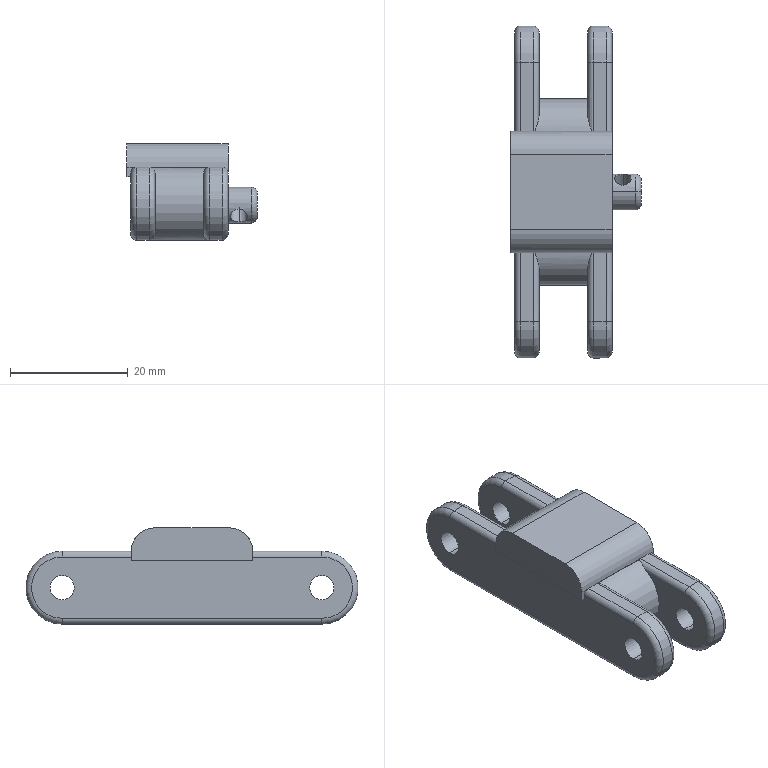Part | SolidWorks | features ICE 7, 3DProfileFeature 2, Fillet 2, Extrusion 1, LPattern 1, Scale 1 | 1 solid | 92 faces | box 22.123 x 56.398 x 16.345 mm | volume 8448 mm3 | plane 46 | cylinder 36 | torus 10 | commonest cylinder face diameters 1.981 x14 12.383 x6 4.127 x4 4.128 x4 2.822 x2 6.09 x2